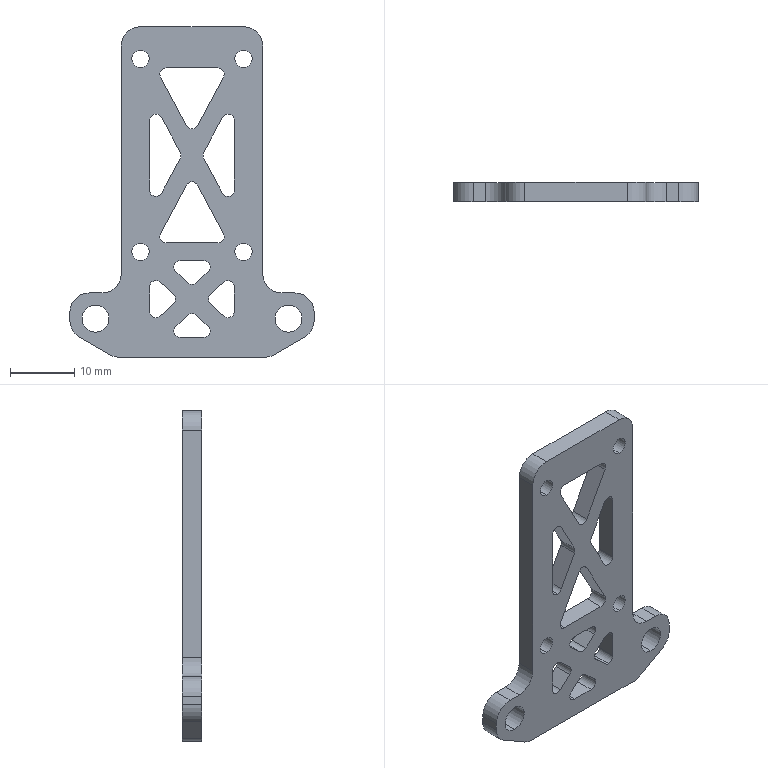Part | SolidWorks | features Fillet 2, Extrusion 1, ICE 1 | 1 solid | 88 faces | box 38 x 3 x 51.4 mm | volume 2836 mm3 | cylinder 52 | plane 36 | commonest cylinder face diameters 2 x30 6 x10 2.7 x8 4.2 x4